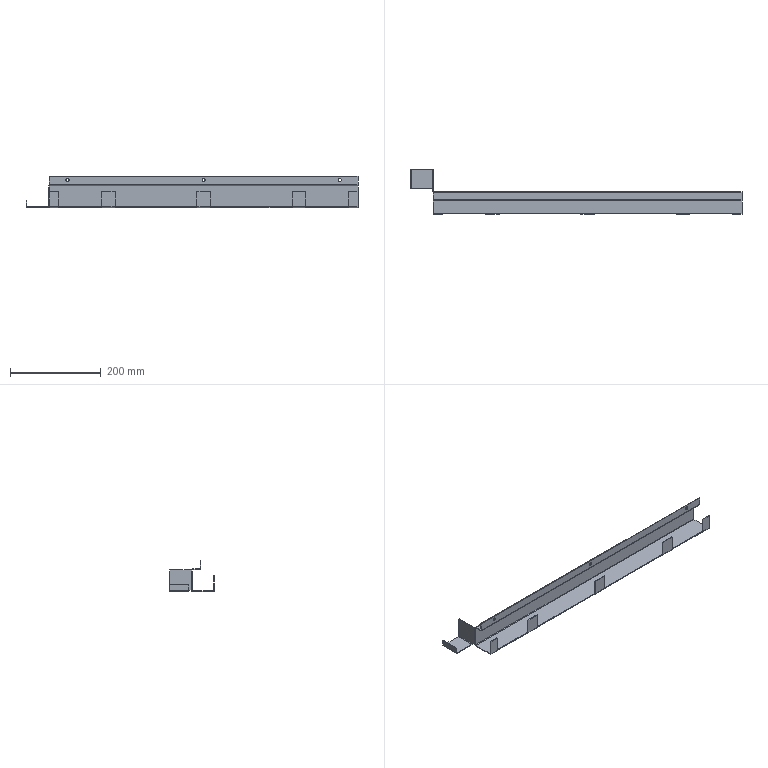Part | STEP file | 1 solid | 103 faces | box 731.5 x 98.5 x 68.5 mm | volume 147735 mm3 | plane 83 | cylinder 20 | commonest cylinder face diameters 2 x7 5 x7 7 x6